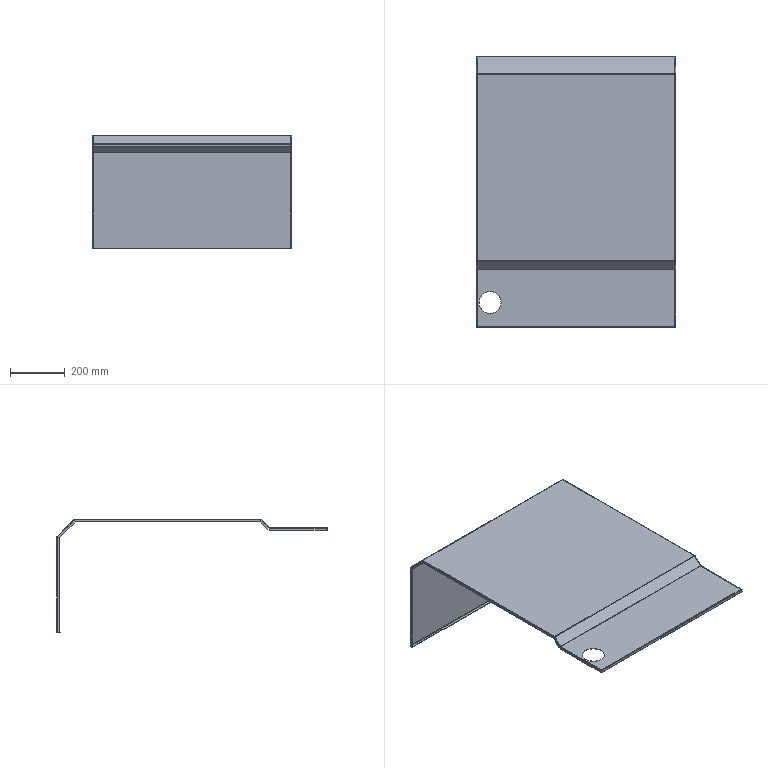Part | STEP file | Inner Lining Plate | 1 solid | 144 faces | box 728 x 988 x 415.5 mm | volume 2061913 mm3 | plane 98 | cylinder 34 | spline 12 | commonest cylinder face diameters 1 x16 5 x16 80 x2